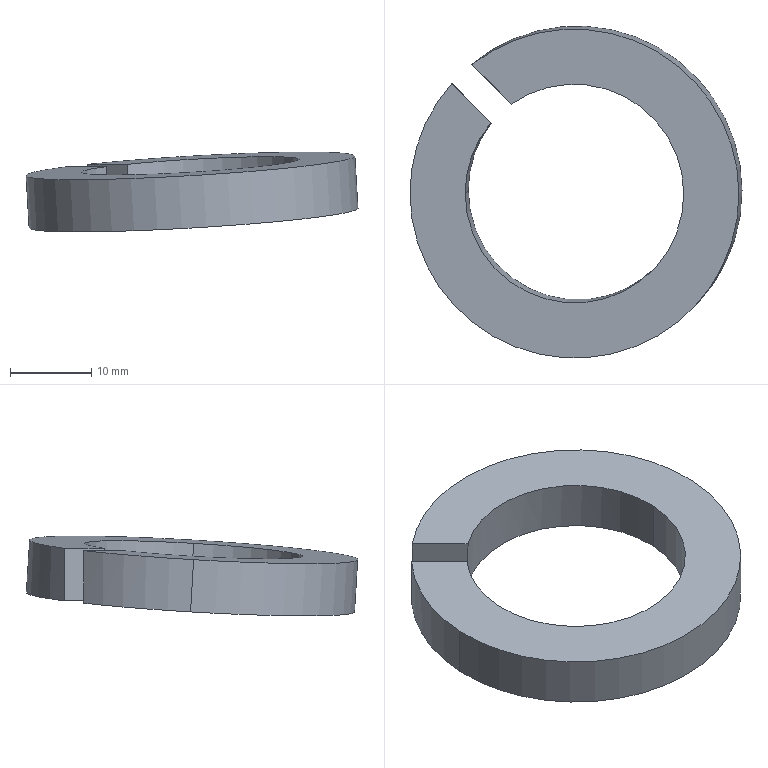Part | SolidWorks | features Boss 1, Cut 1, Extrusion 1, Helix 1, Sweep 1 | 1 solid | 10 faces | box 40.929 x 40.929 x 9.844 mm | volume 4521 mm3 | cylinder 6 | plane 4 | commonest cylinder face diameters 27 x3 40.618 x3
STEP:
#1=CARTESIAN_POINT('',(-13.514,-0.03765,-0.1695));
#2=VERTEX_POINT('',#1);
#3=CARTESIAN_POINT('',(13.438,-0.03765,1.435));
#4=VERTEX_POINT('',#3);
#5=CARTESIAN_POINT('',(-0.03765,-0.03765,0.6326));
#6=DIRECTION('',(-0.05931,-0.05931,0.9965));
#7=DIRECTION('',(0.9982,0.,0.05942));
#8=AXIS2_PLACEMENT_3D('',#5,#6,#7);
#9=CIRCLE('',#8,13.5);
#10=EDGE_CURVE('',#2,#4,#9,.T.);
#11=ORIENTED_EDGE('',*,*,#10,.F.);
#12=CARTESIAN_POINT('',(-13.897,-0.4208,6.268));
#13=VERTEX_POINT('',#12);
#14=CARTESIAN_POINT('',(-13.514,-0.03765,-0.1695));
#15=DIRECTION('',(-0.05931,-0.05931,0.9965));
#16=VECTOR('',#15,1000.);
#17=LINE('',#14,#16);
#18=EDGE_CURVE('',#2,#13,#17,.T.);
#19=ORIENTED_EDGE('',*,*,#18,.T.);
#20=CARTESIAN_POINT('',(13.055,-0.4208,7.872));
#21=VERTEX_POINT('',#20);
#22=CARTESIAN_POINT('',(-0.4208,-0.4208,7.07));
#23=DIRECTION('',(-0.05931,-0.05931,0.9965));
#24=DIRECTION('',(0.9982,0.,0.05942));
#25=AXIS2_PLACEMENT_3D('',#22,#23,#24);
#26=CIRCLE('',#25,13.5);
#27=EDGE_CURVE('',#13,#21,#26,.T.);
#28=ORIENTED_EDGE('',*,*,#27,.T.);
#29=CARTESIAN_POINT('',(13.438,-0.03765,1.435));
#30=DIRECTION('',(-0.05931,-0.05931,0.9965));
#31=VECTOR('',#30,1000.);
#32=LINE('',#29,#31);
#33=EDGE_CURVE('',#4,#21,#32,.T.);
#34=ORIENTED_EDGE('',*,*,#33,.F.);
#35=EDGE_LOOP('',(#11,#19,#28,#34));
#36=FACE_OUTER_BOUND('',#35,.T.);
#37=CARTESIAN_POINT('',(-0.03765,-0.03765,0.6326));
#38=DIRECTION('',(-0.05931,-0.05931,0.9965));
#39=DIRECTION('',(0.9982,0.,0.05942));
#40=AXIS2_PLACEMENT_3D('',#37,#38,#39);
#41=CYLINDRICAL_SURFACE('',#40,13.5);
#42=ADVANCED_FACE('',(#36),#41,.F.);
#43=CARTESIAN_POINT('',(-8.262,10.667,0.7802));
#44=VERTEX_POINT('',#43);
#45=CARTESIAN_POINT('',(-0.03765,-0.03765,0.6326));
#46=DIRECTION('',(-0.05931,-0.05931,0.9965));
#47=DIRECTION('',(0.9982,0.,0.05942));
#48=AXIS2_PLACEMENT_3D('',#45,#46,#47);
#49=CIRCLE('',#48,13.5);
#50=EDGE_CURVE('',#4,#44,#49,.T.);
#51=ORIENTED_EDGE('',*,*,#50,.F.);
#52=ORIENTED_EDGE('',*,*,#33,.T.);
#53=CARTESIAN_POINT('',(-8.204,10.608,7.263));
#54=VERTEX_POINT('',#53);
#55=CARTESIAN_POINT('',(-0.4208,-0.4208,7.07));
#56=DIRECTION('',(-0.05931,-0.05931,0.9965));
#57=DIRECTION('',(0.9982,0.,0.05942));
#58=AXIS2_PLACEMENT_3D('',#55,#56,#57);
#59=CIRCLE('',#58,13.5);
#60=EDGE_CURVE('',#21,#54,#59,.T.);
#61=ORIENTED_EDGE('',*,*,#60,.T.);
#62=CARTESIAN_POINT('',(-8.204,10.608,7.263));
#63=CARTESIAN_POINT('',(-8.226,10.63,5.109));
#64=CARTESIAN_POINT('',(-8.246,10.65,2.948));
#65=CARTESIAN_POINT('',(-8.262,10.667,0.7802));
#66=(BOUNDED_CURVE()B_SPLINE_CURVE(3,(#62,#63,#64,#65),.UNSPECIFIED.,.F.,.F.)B_SPLINE_CURVE_WITH_KNOTS((4,4),(1.399,1.44),.UNSPECIFIED.)CURVE()GEOMETRIC_REPRESENTATION_ITEM()RATIONAL_B_SPLINE_CURVE((1.,0.9999,0.9999,1.))REPRESENTATION_ITEM(''));
#67=EDGE_CURVE('',#54,#44,#66,.T.);
#68=ORIENTED_EDGE('',*,*,#67,.T.);
#69=EDGE_LOOP('',(#51,#52,#61,#68));
#70=FACE_OUTER_BOUND('',#69,.T.);
#71=CARTESIAN_POINT('',(-0.03765,-0.03765,0.6326));
#72=DIRECTION('',(-0.05931,-0.05931,0.9965));
#73=DIRECTION('',(0.9982,0.,0.05942));
#74=AXIS2_PLACEMENT_3D('',#71,#72,#73);
#75=CYLINDRICAL_SURFACE('',#74,13.5);
#76=ADVANCED_FACE('',(#70),#75,.F.);
#77=CARTESIAN_POINT('',(-15.515,13.111,0.494));
#78=VERTEX_POINT('',#77);
#79=CARTESIAN_POINT('',(-20.311,-0.03765,-0.5741));
#80=VERTEX_POINT('',#79);
#81=CARTESIAN_POINT('',(-0.03765,-0.03765,0.6326));
#82=DIRECTION('',(-0.05931,-0.05931,0.9965));
#83=DIRECTION('',(0.9982,0.,0.05942));
#84=AXIS2_PLACEMENT_3D('',#81,#82,#83);
#85=CIRCLE('',#84,20.309);
#86=EDGE_CURVE('',#78,#80,#85,.T.);
#87=ORIENTED_EDGE('',*,*,#86,.T.);
#88=CARTESIAN_POINT('',(-20.694,-0.4208,5.863));
#89=VERTEX_POINT('',#88);
#90=CARTESIAN_POINT('',(-20.311,-0.03765,-0.5741));
#91=DIRECTION('',(-0.05931,-0.05931,0.9965));
#92=VECTOR('',#91,1000.);
#93=LINE('',#90,#92);
#94=EDGE_CURVE('',#80,#89,#93,.T.);
#95=ORIENTED_EDGE('',*,*,#94,.T.);
#96=CARTESIAN_POINT('',(-15.541,13.137,6.977));
#97=VERTEX_POINT('',#96);
#98=CARTESIAN_POINT('',(-0.4208,-0.4208,7.07));
#99=DIRECTION('',(-0.05931,-0.05931,0.9965));
#100=DIRECTION('',(0.9982,0.,0.05942));
#101=AXIS2_PLACEMENT_3D('',#98,#99,#100);
#102=CIRCLE('',#101,20.309);
#103=EDGE_CURVE('',#97,#89,#102,.T.);
#104=ORIENTED_EDGE('',*,*,#103,.F.);
#105=CARTESIAN_POINT('',(-15.515,13.111,0.494));
#106=CARTESIAN_POINT('',(-15.525,13.121,2.653));
#107=CARTESIAN_POINT('',(-15.534,13.13,4.814));
#108=CARTESIAN_POINT('',(-15.541,13.137,6.977));
#109=(BOUNDED_CURVE()B_SPLINE_CURVE(3,(#105,#106,#107,#108),.UNSPECIFIED.,.F.,.F.)B_SPLINE_CURVE_WITH_KNOTS((4,4),(4.631,4.658),.UNSPECIFIED.)CURVE()GEOMETRIC_REPRESENTATION_ITEM()RATIONAL_B_SPLINE_CURVE((1.,0.9999,0.9999,1.))REPRESENTATION_ITEM(''));
#110=EDGE_CURVE('',#78,#97,#109,.T.);
#111=ORIENTED_EDGE('',*,*,#110,.F.);
#112=EDGE_LOOP('',(#87,#95,#104,#111));
#113=FACE_OUTER_BOUND('',#112,.T.);
#114=CARTESIAN_POINT('',(-0.03765,-0.03765,0.6326));
#115=DIRECTION('',(-0.05931,-0.05931,0.9965));
#116=DIRECTION('',(0.9982,0.,0.05942));
#117=AXIS2_PLACEMENT_3D('',#114,#115,#116);
#118=CYLINDRICAL_SURFACE('',#117,20.309);
#119=ADVANCED_FACE('',(#113),#118,.T.);
#120=ORIENTED_EDGE('',*,*,#94,.F.);
#121=CARTESIAN_POINT('',(20.235,-0.03765,1.839));
#122=VERTEX_POINT('',#121);
#123=CARTESIAN_POINT('',(-0.03765,-0.03765,0.6326));
#124=DIRECTION('',(-0.05931,-0.05931,0.9965));
#125=DIRECTION('',(0.9982,0.,0.05942));
#126=AXIS2_PLACEMENT_3D('',#123,#124,#125);
#127=CIRCLE('',#126,20.309);
#128=EDGE_CURVE('',#80,#122,#127,.T.);
#129=ORIENTED_EDGE('',*,*,#128,.T.);
#130=CARTESIAN_POINT('',(19.852,-0.4208,8.277));
#131=VERTEX_POINT('',#130);
#132=CARTESIAN_POINT('',(20.235,-0.03765,1.839));
#133=DIRECTION('',(-0.05931,-0.05931,0.9965));
#134=VECTOR('',#133,1000.);
#135=LINE('',#132,#134);
#136=EDGE_CURVE('',#122,#131,#135,.T.);
#137=ORIENTED_EDGE('',*,*,#136,.T.);
#138=CARTESIAN_POINT('',(-0.4208,-0.4208,7.07));
#139=DIRECTION('',(-0.05931,-0.05931,0.9965));
#140=DIRECTION('',(0.9982,0.,0.05942));
#141=AXIS2_PLACEMENT_3D('',#138,#139,#140);
#142=CIRCLE('',#141,20.309);
#143=EDGE_CURVE('',#89,#131,#142,.T.);
#144=ORIENTED_EDGE('',*,*,#143,.F.);
#145=EDGE_LOOP('',(#120,#129,#137,#144));
#146=FACE_OUTER_BOUND('',#145,.T.);
#147=CARTESIAN_POINT('',(-0.03765,-0.03765,0.6326));
#148=DIRECTION('',(-0.05931,-0.05931,0.9965));
#149=DIRECTION('',(0.9982,0.,0.05942));
#150=AXIS2_PLACEMENT_3D('',#147,#148,#149);
#151=CYLINDRICAL_SURFACE('',#150,20.309);
#152=ADVANCED_FACE('',(#146),#151,.T.);
#153=ORIENTED_EDGE('',*,*,#136,.F.);
#154=CARTESIAN_POINT('',(-13.104,15.509,0.7802));
#155=VERTEX_POINT('',#154);
#156=CARTESIAN_POINT('',(-0.03765,-0.03765,0.6326));
#157=DIRECTION('',(-0.05931,-0.05931,0.9965));
#158=DIRECTION('',(0.9982,0.,0.05942));
#159=AXIS2_PLACEMENT_3D('',#156,#157,#158);
#160=CIRCLE('',#159,20.309);
#161=EDGE_CURVE('',#122,#155,#160,.T.);
#162=ORIENTED_EDGE('',*,*,#161,.T.);
#163=CARTESIAN_POINT('',(-13.066,15.47,7.263));
#164=VERTEX_POINT('',#163);
#165=CARTESIAN_POINT('',(-13.066,15.47,7.263));
#166=CARTESIAN_POINT('',(-13.08,15.485,5.105));
#167=CARTESIAN_POINT('',(-13.093,15.497,2.944));
#168=CARTESIAN_POINT('',(-13.104,15.509,0.7802));
#169=(BOUNDED_CURVE()B_SPLINE_CURVE(3,(#165,#166,#167,#168),.UNSPECIFIED.,.F.,.F.)B_SPLINE_CURVE_WITH_KNOTS((4,4),(1.457,1.484),.UNSPECIFIED.)CURVE()GEOMETRIC_REPRESENTATION_ITEM()RATIONAL_B_SPLINE_CURVE((1.,0.9999,0.9999,1.))REPRESENTATION_ITEM(''));
#170=EDGE_CURVE('',#164,#155,#169,.T.);
#171=ORIENTED_EDGE('',*,*,#170,.F.);
#172=CARTESIAN_POINT('',(-0.4208,-0.4208,7.07));
#173=DIRECTION('',(-0.05931,-0.05931,0.9965));
#174=DIRECTION('',(0.9982,0.,0.05942));
#175=AXIS2_PLACEMENT_3D('',#172,#173,#174);
#176=CIRCLE('',#175,20.309);
#177=EDGE_CURVE('',#131,#164,#176,.T.);
#178=ORIENTED_EDGE('',*,*,#177,.F.);
#179=EDGE_LOOP('',(#153,#162,#171,#178));
#180=FACE_OUTER_BOUND('',#179,.T.);
#181=CARTESIAN_POINT('',(-0.03765,-0.03765,0.6326));
#182=DIRECTION('',(-0.05931,-0.05931,0.9965));
#183=DIRECTION('',(0.9982,0.,0.05942));
#184=AXIS2_PLACEMENT_3D('',#181,#182,#183);
#185=CYLINDRICAL_SURFACE('',#184,20.309);
#186=ADVANCED_FACE('',(#180),#185,.T.);
#187=ORIENTED_EDGE('',*,*,#86,.F.);
#188=CARTESIAN_POINT('',(-10.676,8.272,0.494));
#189=VERTEX_POINT('',#188);
#190=CARTESIAN_POINT('',(-1.202,-1.202,0.494));
#191=DIRECTION('',(0.7071,-0.7071,0.));
#192=VECTOR('',#191,1000.);
#193=LINE('',#190,#192);
#194=EDGE_CURVE('',#78,#189,#193,.T.);
#195=ORIENTED_EDGE('',*,*,#194,.T.);
#196=CARTESIAN_POINT('',(-0.03765,-0.03765,0.6326));
#197=DIRECTION('',(-0.05931,-0.05931,0.9965));
#198=DIRECTION('',(0.9982,0.,0.05942));
#199=AXIS2_PLACEMENT_3D('',#196,#197,#198);
#200=CIRCLE('',#199,13.5);
#201=EDGE_CURVE('',#189,#2,#200,.T.);
#202=ORIENTED_EDGE('',*,*,#201,.T.);
#203=ORIENTED_EDGE('',*,*,#10,.T.);
#204=ORIENTED_EDGE('',*,*,#50,.T.);
#205=CARTESIAN_POINT('',(1.202,1.202,0.7802));
#206=DIRECTION('',(-0.7071,0.7071,0.));
#207=VECTOR('',#206,1000.);
#208=LINE('',#205,#207);
#209=EDGE_CURVE('',#44,#155,#208,.T.);
#210=ORIENTED_EDGE('',*,*,#209,.T.);
#211=ORIENTED_EDGE('',*,*,#161,.F.);
#212=ORIENTED_EDGE('',*,*,#128,.F.);
#213=EDGE_LOOP('',(#187,#195,#202,#203,#204,#210,#211,#212));
#214=FACE_OUTER_BOUND('',#213,.T.);
#215=CARTESIAN_POINT('',(-0.03765,-0.03765,0.6326));
#216=DIRECTION('',(-0.05931,-0.05931,0.9965));
#217=DIRECTION('',(0.9982,0.,0.05942));
#218=AXIS2_PLACEMENT_3D('',#215,#216,#217);
#219=PLANE('',#218);
#220=ADVANCED_FACE('',(#214),#219,.F.);
#221=ORIENTED_EDGE('',*,*,#18,.F.);
#222=ORIENTED_EDGE('',*,*,#201,.F.);
#223=CARTESIAN_POINT('',(-10.716,8.312,6.977));
#224=VERTEX_POINT('',#223);
#225=CARTESIAN_POINT('',(-10.676,8.272,0.494));
#226=CARTESIAN_POINT('',(-10.692,8.288,2.65));
#227=CARTESIAN_POINT('',(-10.705,8.301,4.812));
#228=CARTESIAN_POINT('',(-10.716,8.312,6.977));
#229=(BOUNDED_CURVE()B_SPLINE_CURVE(3,(#225,#226,#227,#228),.UNSPECIFIED.,.F.,.F.)B_SPLINE_CURVE_WITH_KNOTS((4,4),(4.59,4.63),.UNSPECIFIED.)CURVE()GEOMETRIC_REPRESENTATION_ITEM()RATIONAL_B_SPLINE_CURVE((1.,0.9999,0.9999,1.))REPRESENTATION_ITEM(''));
#230=EDGE_CURVE('',#189,#224,#229,.T.);
#231=ORIENTED_EDGE('',*,*,#230,.T.);
#232=CARTESIAN_POINT('',(-0.4208,-0.4208,7.07));
#233=DIRECTION('',(-0.05931,-0.05931,0.9965));
#234=DIRECTION('',(0.9982,0.,0.05942));
#235=AXIS2_PLACEMENT_3D('',#232,#233,#234);
#236=CIRCLE('',#235,13.5);
#237=EDGE_CURVE('',#224,#13,#236,.T.);
#238=ORIENTED_EDGE('',*,*,#237,.T.);
#239=EDGE_LOOP('',(#221,#222,#231,#238));
#240=FACE_OUTER_BOUND('',#239,.T.);
#241=CARTESIAN_POINT('',(-0.03765,-0.03765,0.6326));
#242=DIRECTION('',(-0.05931,-0.05931,0.9965));
#243=DIRECTION('',(0.9982,0.,0.05942));
#244=AXIS2_PLACEMENT_3D('',#241,#242,#243);
#245=CYLINDRICAL_SURFACE('',#244,13.5);
#246=ADVANCED_FACE('',(#240),#245,.F.);
#247=CARTESIAN_POINT('',(-15.542,13.138,6.977));
#248=DIRECTION('',(0.7071,-0.7071,0.));
#249=VECTOR('',#248,1000.);
#250=LINE('',#247,#249);
#251=EDGE_CURVE('',#97,#224,#250,.T.);
#252=ORIENTED_EDGE('',*,*,#251,.F.);
#253=ORIENTED_EDGE('',*,*,#103,.T.);
#254=ORIENTED_EDGE('',*,*,#143,.T.);
#255=ORIENTED_EDGE('',*,*,#177,.T.);
#256=CARTESIAN_POINT('',(-13.138,15.542,7.263));
#257=DIRECTION('',(-0.7071,0.7071,0.));
#258=VECTOR('',#257,1000.);
#259=LINE('',#256,#258);
#260=EDGE_CURVE('',#54,#164,#259,.T.);
#261=ORIENTED_EDGE('',*,*,#260,.F.);
#262=ORIENTED_EDGE('',*,*,#60,.F.);
#263=ORIENTED_EDGE('',*,*,#27,.F.);
#264=ORIENTED_EDGE('',*,*,#237,.F.);
#265=EDGE_LOOP('',(#252,#253,#254,#255,#261,#262,#263,#264));
#266=FACE_OUTER_BOUND('',#265,.T.);
#267=CARTESIAN_POINT('',(-14.34,14.341,7.12));
#268=DIRECTION('',(-0.05931,-0.05931,0.9965));
#269=DIRECTION('',(0.9982,0.,0.05942));
#270=AXIS2_PLACEMENT_3D('',#267,#268,#269);
#271=PLANE('',#270);
#272=ADVANCED_FACE('',(#266),#271,.T.);
#273=ORIENTED_EDGE('',*,*,#170,.T.);
#274=ORIENTED_EDGE('',*,*,#209,.F.);
#275=ORIENTED_EDGE('',*,*,#67,.F.);
#276=ORIENTED_EDGE('',*,*,#260,.T.);
#277=EDGE_LOOP('',(#273,#274,#275,#276));
#278=FACE_OUTER_BOUND('',#277,.T.);
#279=CARTESIAN_POINT('',(-34.049,36.453,-1.071));
#280=DIRECTION('',(0.7071,0.7071,0.));
#281=DIRECTION('',(-0.7071,0.7071,0.));
#282=AXIS2_PLACEMENT_3D('',#279,#280,#281);
#283=PLANE('',#282);
#284=ADVANCED_FACE('',(#278),#283,.F.);
#285=ORIENTED_EDGE('',*,*,#110,.T.);
#286=ORIENTED_EDGE('',*,*,#251,.T.);
#287=ORIENTED_EDGE('',*,*,#230,.F.);
#288=ORIENTED_EDGE('',*,*,#194,.F.);
#289=EDGE_LOOP('',(#285,#286,#287,#288));
#290=FACE_OUTER_BOUND('',#289,.T.);
#291=CARTESIAN_POINT('',(-1.451,-0.9529,-1.071));
#292=DIRECTION('',(-0.7071,-0.7071,0.));
#293=DIRECTION('',(0.7071,-0.7071,0.));
#294=AXIS2_PLACEMENT_3D('',#291,#292,#293);
#295=PLANE('',#294);
#296=ADVANCED_FACE('',(#290),#295,.F.);
#297=CLOSED_SHELL('',(#42,#76,#119,#152,#186,#220,#246,#272,#284,#296));
#298=MANIFOLD_SOLID_BREP('',#297);
#299=CARTESIAN_POINT('',(0.,0.,0.));
#300=DIRECTION('',(0.,0.,1.));
#301=DIRECTION('',(1.,0.,0.));
#302=AXIS2_PLACEMENT_3D('',#299,#300,#301);
#303=(LENGTH_UNIT()NAMED_UNIT(*)SI_UNIT(.MILLI.,.METRE.));
#304=UNCERTAINTY_MEASURE_WITH_UNIT(LENGTH_MEASURE(0.00001),#303,'','');
#305=(NAMED_UNIT(*)PLANE_ANGLE_UNIT()SI_UNIT($,.RADIAN.));
#306=(NAMED_UNIT(*)SI_UNIT($,.STERADIAN.)SOLID_ANGLE_UNIT());
#307=(GEOMETRIC_REPRESENTATION_CONTEXT(3)GLOBAL_UNCERTAINTY_ASSIGNED_CONTEXT((#304))GLOBAL_UNIT_ASSIGNED_CONTEXT((#303,#305,#306))REPRESENTATION_CONTEXT('',''));
#308=ADVANCED_BREP_SHAPE_REPRESENTATION('',(#298,#302),#307);